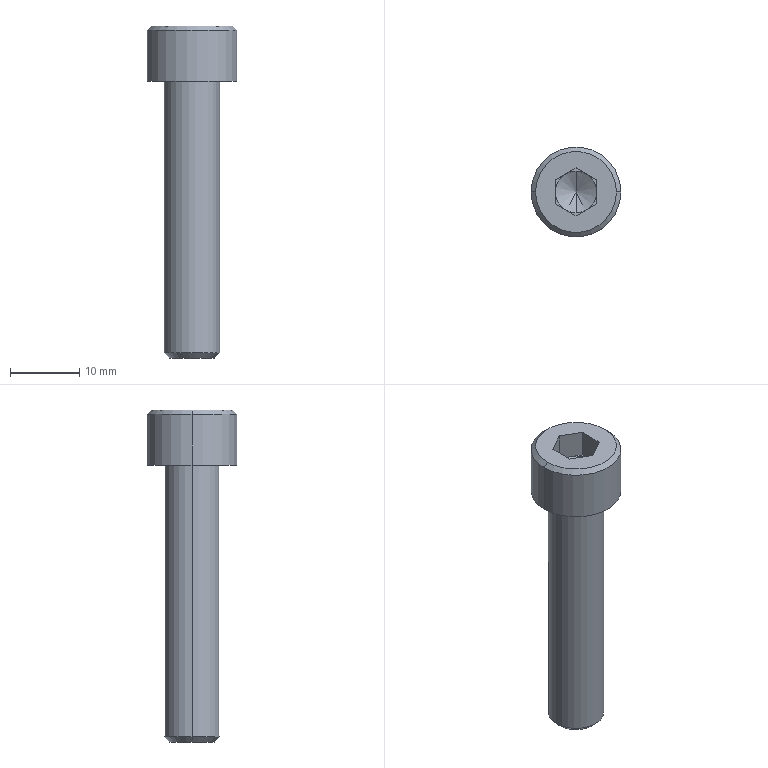Part | SolidWorks | features Chamfer 2, ICE 2, RevCut 1, Revolution 1 | 1 solid | 25 faces | box 13 x 13 x 48 mm | volume 2916 mm3 | plane 15 | cone 6 | cylinder 4 | commonest cylinder face diameters 8 x2 13 x2
STEP:
#1=CARTESIAN_POINT('',(-3.233,0.,-40.));
#2=VERTEX_POINT('',#1);
#3=CARTESIAN_POINT('',(3.233,0.,-40.));
#4=VERTEX_POINT('',#3);
#5=CARTESIAN_POINT('',(0.,0.,-40.));
#6=DIRECTION('',(0.,0.,-1.));
#7=DIRECTION('',(-1.,0.,0.));
#8=AXIS2_PLACEMENT_3D('',#5,#6,#7);
#9=CIRCLE('',#8,3.233);
#10=EDGE_CURVE('',#2,#4,#9,.T.);
#11=ORIENTED_EDGE('',*,*,#10,.F.);
#12=CARTESIAN_POINT('',(-4.,0.,-39.233));
#13=VERTEX_POINT('',#12);
#14=CARTESIAN_POINT('',(-3.233,0.,-40.));
#15=DIRECTION('',(-0.7071,0.,0.7071));
#16=VECTOR('',#15,1000.);
#17=LINE('',#14,#16);
#18=EDGE_CURVE('',#2,#13,#17,.T.);
#19=ORIENTED_EDGE('',*,*,#18,.T.);
#20=CARTESIAN_POINT('',(4.,0.,-39.233));
#21=VERTEX_POINT('',#20);
#22=CARTESIAN_POINT('',(0.,0.,-39.233));
#23=DIRECTION('',(0.,0.,1.));
#24=DIRECTION('',(-1.,0.,0.));
#25=AXIS2_PLACEMENT_3D('',#22,#23,#24);
#26=CIRCLE('',#25,4.);
#27=EDGE_CURVE('',#21,#13,#26,.T.);
#28=ORIENTED_EDGE('',*,*,#27,.F.);
#29=CARTESIAN_POINT('',(3.233,0.,-40.));
#30=DIRECTION('',(0.7071,0.,0.7071));
#31=VECTOR('',#30,1000.);
#32=LINE('',#29,#31);
#33=EDGE_CURVE('',#4,#21,#32,.T.);
#34=ORIENTED_EDGE('',*,*,#33,.F.);
#35=EDGE_LOOP('',(#11,#19,#28,#34));
#36=FACE_OUTER_BOUND('',#35,.T.);
#37=CARTESIAN_POINT('',(0.,0.,-40.));
#38=DIRECTION('',(0.,0.,1.));
#39=DIRECTION('',(1.,0.,0.));
#40=AXIS2_PLACEMENT_3D('',#37,#38,#39);
#41=CONICAL_SURFACE('',#40,3.233,0.7854);
#42=ADVANCED_FACE('',(#36),#41,.T.);
#43=CARTESIAN_POINT('',(5.85,0.,8.));
#44=VERTEX_POINT('',#43);
#45=CARTESIAN_POINT('',(-5.85,0.,8.));
#46=VERTEX_POINT('',#45);
#47=CARTESIAN_POINT('',(0.,0.,8.));
#48=DIRECTION('',(0.,0.,1.));
#49=DIRECTION('',(1.,0.,0.));
#50=AXIS2_PLACEMENT_3D('',#47,#48,#49);
#51=CIRCLE('',#50,5.85);
#52=EDGE_CURVE('',#44,#46,#51,.T.);
#53=ORIENTED_EDGE('',*,*,#52,.F.);
#54=CARTESIAN_POINT('',(6.5,0.,7.35));
#55=VERTEX_POINT('',#54);
#56=CARTESIAN_POINT('',(5.85,0.,8.));
#57=DIRECTION('',(0.7071,0.,-0.7071));
#58=VECTOR('',#57,1000.);
#59=LINE('',#56,#58);
#60=EDGE_CURVE('',#44,#55,#59,.T.);
#61=ORIENTED_EDGE('',*,*,#60,.T.);
#62=CARTESIAN_POINT('',(-6.5,0.,7.35));
#63=VERTEX_POINT('',#62);
#64=CARTESIAN_POINT('',(0.,0.,7.35));
#65=DIRECTION('',(0.,0.,-1.));
#66=DIRECTION('',(1.,0.,0.));
#67=AXIS2_PLACEMENT_3D('',#64,#65,#66);
#68=CIRCLE('',#67,6.5);
#69=EDGE_CURVE('',#63,#55,#68,.T.);
#70=ORIENTED_EDGE('',*,*,#69,.F.);
#71=CARTESIAN_POINT('',(-5.85,0.,8.));
#72=DIRECTION('',(-0.7071,0.,-0.7071));
#73=VECTOR('',#72,1000.);
#74=LINE('',#71,#73);
#75=EDGE_CURVE('',#46,#63,#74,.T.);
#76=ORIENTED_EDGE('',*,*,#75,.F.);
#77=EDGE_LOOP('',(#53,#61,#70,#76));
#78=FACE_OUTER_BOUND('',#77,.T.);
#79=CARTESIAN_POINT('',(0.,0.,8.));
#80=DIRECTION('',(0.,0.,-1.));
#81=DIRECTION('',(-1.,0.,0.));
#82=AXIS2_PLACEMENT_3D('',#79,#80,#81);
#83=CONICAL_SURFACE('',#82,5.85,0.7854);
#84=ADVANCED_FACE('',(#78),#83,.T.);
#85=CARTESIAN_POINT('',(0.,0.,2.268));
#86=VERTEX_POINT('',#85);
#87=CARTESIAN_POINT('',(0.,-3.,4.));
#88=VERTEX_POINT('',#87);
#89=CARTESIAN_POINT('',(0.,0.,2.268));
#90=DIRECTION('',(0.,-0.866,0.5));
#91=VECTOR('',#90,1000.);
#92=LINE('',#89,#91);
#93=EDGE_CURVE('',#86,#88,#92,.T.);
#94=ORIENTED_EDGE('',*,*,#93,.F.);
#95=CARTESIAN_POINT('',(0.,3.,4.));
#96=VERTEX_POINT('',#95);
#97=CARTESIAN_POINT('',(0.,0.,2.268));
#98=DIRECTION('',(0.,0.866,0.5));
#99=VECTOR('',#98,1000.);
#100=LINE('',#97,#99);
#101=EDGE_CURVE('',#86,#96,#100,.T.);
#102=ORIENTED_EDGE('',*,*,#101,.T.);
#103=CARTESIAN_POINT('',(-1.5,2.598,4.));
#104=VERTEX_POINT('',#103);
#105=CARTESIAN_POINT('',(0.,0.,4.));
#106=DIRECTION('',(0.,0.,-1.));
#107=DIRECTION('',(0.,1.,0.));
#108=AXIS2_PLACEMENT_3D('',#105,#106,#107);
#109=CIRCLE('',#108,3.);
#110=EDGE_CURVE('',#104,#96,#109,.T.);
#111=ORIENTED_EDGE('',*,*,#110,.F.);
#112=CARTESIAN_POINT('',(-3.,0.,4.));
#113=VERTEX_POINT('',#112);
#114=CARTESIAN_POINT('',(0.,0.,4.));
#115=DIRECTION('',(0.,0.,-1.));
#116=DIRECTION('',(0.,1.,0.));
#117=AXIS2_PLACEMENT_3D('',#114,#115,#116);
#118=CIRCLE('',#117,3.);
#119=EDGE_CURVE('',#113,#104,#118,.T.);
#120=ORIENTED_EDGE('',*,*,#119,.F.);
#121=CARTESIAN_POINT('',(-1.5,-2.598,4.));
#122=VERTEX_POINT('',#121);
#123=CARTESIAN_POINT('',(0.,0.,4.));
#124=DIRECTION('',(0.,0.,-1.));
#125=DIRECTION('',(0.,1.,0.));
#126=AXIS2_PLACEMENT_3D('',#123,#124,#125);
#127=CIRCLE('',#126,3.);
#128=EDGE_CURVE('',#122,#113,#127,.T.);
#129=ORIENTED_EDGE('',*,*,#128,.F.);
#130=CARTESIAN_POINT('',(0.,0.,4.));
#131=DIRECTION('',(0.,0.,-1.));
#132=DIRECTION('',(0.,1.,0.));
#133=AXIS2_PLACEMENT_3D('',#130,#131,#132);
#134=CIRCLE('',#133,3.);
#135=EDGE_CURVE('',#88,#122,#134,.T.);
#136=ORIENTED_EDGE('',*,*,#135,.F.);
#137=EDGE_LOOP('',(#94,#102,#111,#120,#129,#136));
#138=FACE_OUTER_BOUND('',#137,.T.);
#139=CARTESIAN_POINT('',(0.,0.,1002.268));
#140=DIRECTION('',(0.,0.,1.));
#141=DIRECTION('',(0.,-1.,0.));
#142=AXIS2_PLACEMENT_3D('',#139,#140,#141);
#143=CONICAL_SURFACE('',#142,1732.051,1.047);
#144=ADVANCED_FACE('',(#138),#143,.F.);
#145=ORIENTED_EDGE('',*,*,#27,.T.);
#146=CARTESIAN_POINT('',(-4.,0.,0.));
#147=VERTEX_POINT('',#146);
#148=CARTESIAN_POINT('',(-4.,0.,-40.));
#149=DIRECTION('',(0.,0.,1.));
#150=VECTOR('',#149,1000.);
#151=LINE('',#148,#150);
#152=EDGE_CURVE('',#13,#147,#151,.T.);
#153=ORIENTED_EDGE('',*,*,#152,.T.);
#154=CARTESIAN_POINT('',(4.,0.,0.));
#155=VERTEX_POINT('',#154);
#156=CARTESIAN_POINT('',(0.,0.,0.));
#157=DIRECTION('',(0.,0.,-1.));
#158=DIRECTION('',(-1.,0.,0.));
#159=AXIS2_PLACEMENT_3D('',#156,#157,#158);
#160=CIRCLE('',#159,4.);
#161=EDGE_CURVE('',#147,#155,#160,.T.);
#162=ORIENTED_EDGE('',*,*,#161,.T.);
#163=CARTESIAN_POINT('',(4.,0.,-40.));
#164=DIRECTION('',(0.,0.,1.));
#165=VECTOR('',#164,1000.);
#166=LINE('',#163,#165);
#167=EDGE_CURVE('',#21,#155,#166,.T.);
#168=ORIENTED_EDGE('',*,*,#167,.F.);
#169=EDGE_LOOP('',(#145,#153,#162,#168));
#170=FACE_OUTER_BOUND('',#169,.T.);
#171=CARTESIAN_POINT('',(0.,0.,-40.));
#172=DIRECTION('',(0.,0.,1.));
#173=DIRECTION('',(1.,0.,0.));
#174=AXIS2_PLACEMENT_3D('',#171,#172,#173);
#175=CYLINDRICAL_SURFACE('',#174,4.);
#176=ADVANCED_FACE('',(#170),#175,.T.);
#177=CARTESIAN_POINT('',(6.5,0.,0.));
#178=VERTEX_POINT('',#177);
#179=CARTESIAN_POINT('',(-6.5,0.,0.));
#180=VERTEX_POINT('',#179);
#181=CARTESIAN_POINT('',(0.,0.,0.));
#182=DIRECTION('',(0.,0.,1.));
#183=DIRECTION('',(1.,0.,0.));
#184=AXIS2_PLACEMENT_3D('',#181,#182,#183);
#185=CIRCLE('',#184,6.5);
#186=EDGE_CURVE('',#178,#180,#185,.T.);
#187=ORIENTED_EDGE('',*,*,#186,.T.);
#188=CARTESIAN_POINT('',(-6.5,0.,0.));
#189=DIRECTION('',(0.,0.,1.));
#190=VECTOR('',#189,1000.);
#191=LINE('',#188,#190);
#192=EDGE_CURVE('',#180,#63,#191,.T.);
#193=ORIENTED_EDGE('',*,*,#192,.T.);
#194=ORIENTED_EDGE('',*,*,#69,.T.);
#195=CARTESIAN_POINT('',(6.5,0.,0.));
#196=DIRECTION('',(0.,0.,1.));
#197=VECTOR('',#196,1000.);
#198=LINE('',#195,#197);
#199=EDGE_CURVE('',#178,#55,#198,.T.);
#200=ORIENTED_EDGE('',*,*,#199,.F.);
#201=EDGE_LOOP('',(#187,#193,#194,#200));
#202=FACE_OUTER_BOUND('',#201,.T.);
#203=CARTESIAN_POINT('',(0.,0.,0.));
#204=DIRECTION('',(0.,0.,1.));
#205=DIRECTION('',(1.,0.,0.));
#206=AXIS2_PLACEMENT_3D('',#203,#204,#205);
#207=CYLINDRICAL_SURFACE('',#206,6.5);
#208=ADVANCED_FACE('',(#202),#207,.T.);
#209=CARTESIAN_POINT('',(3.,1.732,4.));
#210=VERTEX_POINT('',#209);
#211=CARTESIAN_POINT('',(1.5,2.598,4.));
#212=VERTEX_POINT('',#211);
#213=CARTESIAN_POINT('',(3.,1.732,4.));
#214=DIRECTION('',(-0.866,0.5,0.));
#215=VECTOR('',#214,1000.);
#216=LINE('',#213,#215);
#217=EDGE_CURVE('',#210,#212,#216,.T.);
#218=ORIENTED_EDGE('',*,*,#217,.T.);
#219=CARTESIAN_POINT('',(3.,0.,4.));
#220=VERTEX_POINT('',#219);
#221=CARTESIAN_POINT('',(0.,0.,4.));
#222=DIRECTION('',(0.,0.,-1.));
#223=DIRECTION('',(0.,1.,0.));
#224=AXIS2_PLACEMENT_3D('',#221,#222,#223);
#225=CIRCLE('',#224,3.);
#226=EDGE_CURVE('',#212,#220,#225,.T.);
#227=ORIENTED_EDGE('',*,*,#226,.T.);
#228=CARTESIAN_POINT('',(3.,-1.732,4.));
#229=DIRECTION('',(0.,1.,0.));
#230=VECTOR('',#229,1000.);
#231=LINE('',#228,#230);
#232=EDGE_CURVE('',#220,#210,#231,.T.);
#233=ORIENTED_EDGE('',*,*,#232,.T.);
#234=EDGE_LOOP('',(#218,#227,#233));
#235=FACE_OUTER_BOUND('',#234,.T.);
#236=CARTESIAN_POINT('',(0.,0.,4.));
#237=DIRECTION('',(0.,0.,1.));
#238=DIRECTION('',(1.,0.,0.));
#239=AXIS2_PLACEMENT_3D('',#236,#237,#238);
#240=PLANE('',#239);
#241=ADVANCED_FACE('',(#235),#240,.T.);
#242=CARTESIAN_POINT('',(3.,-1.732,4.));
#243=VERTEX_POINT('',#242);
#244=CARTESIAN_POINT('',(3.,-1.732,4.));
#245=DIRECTION('',(0.,1.,0.));
#246=VECTOR('',#245,1000.);
#247=LINE('',#244,#246);
#248=EDGE_CURVE('',#243,#220,#247,.T.);
#249=ORIENTED_EDGE('',*,*,#248,.T.);
#250=CARTESIAN_POINT('',(1.5,-2.598,4.));
#251=VERTEX_POINT('',#250);
#252=CARTESIAN_POINT('',(0.,0.,4.));
#253=DIRECTION('',(0.,0.,-1.));
#254=DIRECTION('',(0.,1.,0.));
#255=AXIS2_PLACEMENT_3D('',#252,#253,#254);
#256=CIRCLE('',#255,3.);
#257=EDGE_CURVE('',#220,#251,#256,.T.);
#258=ORIENTED_EDGE('',*,*,#257,.T.);
#259=CARTESIAN_POINT('',(0.,-3.464,4.));
#260=DIRECTION('',(0.866,0.5,0.));
#261=VECTOR('',#260,1000.);
#262=LINE('',#259,#261);
#263=EDGE_CURVE('',#251,#243,#262,.T.);
#264=ORIENTED_EDGE('',*,*,#263,.T.);
#265=EDGE_LOOP('',(#249,#258,#264));
#266=FACE_OUTER_BOUND('',#265,.T.);
#267=CARTESIAN_POINT('',(0.,0.,4.));
#268=DIRECTION('',(0.,0.,1.));
#269=DIRECTION('',(1.,0.,0.));
#270=AXIS2_PLACEMENT_3D('',#267,#268,#269);
#271=PLANE('',#270);
#272=ADVANCED_FACE('',(#266),#271,.T.);
#273=CARTESIAN_POINT('',(0.,-3.464,4.));
#274=VERTEX_POINT('',#273);
#275=CARTESIAN_POINT('',(0.,-3.464,4.));
#276=DIRECTION('',(0.866,0.5,0.));
#277=VECTOR('',#276,1000.);
#278=LINE('',#275,#277);
#279=EDGE_CURVE('',#274,#251,#278,.T.);
#280=ORIENTED_EDGE('',*,*,#279,.T.);
#281=CARTESIAN_POINT('',(0.,0.,4.));
#282=DIRECTION('',(0.,0.,-1.));
#283=DIRECTION('',(0.,1.,0.));
#284=AXIS2_PLACEMENT_3D('',#281,#282,#283);
#285=CIRCLE('',#284,3.);
#286=EDGE_CURVE('',#251,#88,#285,.T.);
#287=ORIENTED_EDGE('',*,*,#286,.T.);
#288=ORIENTED_EDGE('',*,*,#135,.T.);
#289=CARTESIAN_POINT('',(-3.,-1.732,4.));
#290=DIRECTION('',(0.866,-0.5,0.));
#291=VECTOR('',#290,1000.);
#292=LINE('',#289,#291);
#293=EDGE_CURVE('',#122,#274,#292,.T.);
#294=ORIENTED_EDGE('',*,*,#293,.T.);
#295=EDGE_LOOP('',(#280,#287,#288,#294));
#296=FACE_OUTER_BOUND('',#295,.T.);
#297=CARTESIAN_POINT('',(0.,0.,4.));
#298=DIRECTION('',(0.,0.,1.));
#299=DIRECTION('',(1.,0.,0.));
#300=AXIS2_PLACEMENT_3D('',#297,#298,#299);
#301=PLANE('',#300);
#302=ADVANCED_FACE('',(#296),#301,.T.);
#303=CARTESIAN_POINT('',(-3.,-1.732,4.));
#304=VERTEX_POINT('',#303);
#305=CARTESIAN_POINT('',(-3.,-1.732,4.));
#306=DIRECTION('',(0.866,-0.5,0.));
#307=VECTOR('',#306,1000.);
#308=LINE('',#305,#307);
#309=EDGE_CURVE('',#304,#122,#308,.T.);
#310=ORIENTED_EDGE('',*,*,#309,.T.);
#311=ORIENTED_EDGE('',*,*,#128,.T.);
#312=CARTESIAN_POINT('',(-3.,1.732,4.));
#313=DIRECTION('',(0.,-1.,0.));
#314=VECTOR('',#313,1000.);
#315=LINE('',#312,#314);
#316=EDGE_CURVE('',#113,#304,#315,.T.);
#317=ORIENTED_EDGE('',*,*,#316,.T.);
#318=EDGE_LOOP('',(#310,#311,#317));
#319=FACE_OUTER_BOUND('',#318,.T.);
#320=CARTESIAN_POINT('',(0.,0.,4.));
#321=DIRECTION('',(0.,0.,1.));
#322=DIRECTION('',(1.,0.,0.));
#323=AXIS2_PLACEMENT_3D('',#320,#321,#322);
#324=PLANE('',#323);
#325=ADVANCED_FACE('',(#319),#324,.T.);
#326=CARTESIAN_POINT('',(-3.,1.732,4.));
#327=VERTEX_POINT('',#326);
#328=CARTESIAN_POINT('',(-3.,1.732,4.));
#329=DIRECTION('',(0.,-1.,0.));
#330=VECTOR('',#329,1000.);
#331=LINE('',#328,#330);
#332=EDGE_CURVE('',#327,#113,#331,.T.);
#333=ORIENTED_EDGE('',*,*,#332,.T.);
#334=ORIENTED_EDGE('',*,*,#119,.T.);
#335=CARTESIAN_POINT('',(0.,3.464,4.));
#336=DIRECTION('',(-0.866,-0.5,0.));
#337=VECTOR('',#336,1000.);
#338=LINE('',#335,#337);
#339=EDGE_CURVE('',#104,#327,#338,.T.);
#340=ORIENTED_EDGE('',*,*,#339,.T.);
#341=EDGE_LOOP('',(#333,#334,#340));
#342=FACE_OUTER_BOUND('',#341,.T.);
#343=CARTESIAN_POINT('',(0.,0.,4.));
#344=DIRECTION('',(0.,0.,1.));
#345=DIRECTION('',(1.,0.,0.));
#346=AXIS2_PLACEMENT_3D('',#343,#344,#345);
#347=PLANE('',#346);
#348=ADVANCED_FACE('',(#342),#347,.T.);
#349=CARTESIAN_POINT('',(0.,3.464,4.));
#350=VERTEX_POINT('',#349);
#351=CARTESIAN_POINT('',(0.,3.464,4.));
#352=DIRECTION('',(-0.866,-0.5,0.));
#353=VECTOR('',#352,1000.);
#354=LINE('',#351,#353);
#355=EDGE_CURVE('',#350,#104,#354,.T.);
#356=ORIENTED_EDGE('',*,*,#355,.T.);
#357=ORIENTED_EDGE('',*,*,#110,.T.);
#358=CARTESIAN_POINT('',(0.,0.,4.));
#359=DIRECTION('',(0.,0.,-1.));
#360=DIRECTION('',(0.,1.,0.));
#361=AXIS2_PLACEMENT_3D('',#358,#359,#360);
#362=CIRCLE('',#361,3.);
#363=EDGE_CURVE('',#96,#212,#362,.T.);
#364=ORIENTED_EDGE('',*,*,#363,.T.);
#365=CARTESIAN_POINT('',(3.,1.732,4.));
#366=DIRECTION('',(-0.866,0.5,0.));
#367=VECTOR('',#366,1000.);
#368=LINE('',#365,#367);
#369=EDGE_CURVE('',#212,#350,#368,.T.);
#370=ORIENTED_EDGE('',*,*,#369,.T.);
#371=EDGE_LOOP('',(#356,#357,#364,#370));
#372=FACE_OUTER_BOUND('',#371,.T.);
#373=CARTESIAN_POINT('',(0.,0.,4.));
#374=DIRECTION('',(0.,0.,1.));
#375=DIRECTION('',(1.,0.,0.));
#376=AXIS2_PLACEMENT_3D('',#373,#374,#375);
#377=PLANE('',#376);
#378=ADVANCED_FACE('',(#372),#377,.T.);
#379=ORIENTED_EDGE('',*,*,#186,.F.);
#380=CARTESIAN_POINT('',(0.,0.,0.));
#381=DIRECTION('',(0.,0.,1.));
#382=DIRECTION('',(1.,0.,0.));
#383=AXIS2_PLACEMENT_3D('',#380,#381,#382);
#384=CIRCLE('',#383,6.5);
#385=EDGE_CURVE('',#180,#178,#384,.T.);
#386=ORIENTED_EDGE('',*,*,#385,.F.);
#387=EDGE_LOOP('',(#379,#386));
#388=FACE_OUTER_BOUND('',#387,.T.);
#389=CARTESIAN_POINT('',(0.,0.,0.));
#390=DIRECTION('',(0.,0.,-1.));
#391=DIRECTION('',(-1.,0.,0.));
#392=AXIS2_PLACEMENT_3D('',#389,#390,#391);
#393=CIRCLE('',#392,4.);
#394=EDGE_CURVE('',#155,#147,#393,.T.);
#395=ORIENTED_EDGE('',*,*,#394,.F.);
#396=ORIENTED_EDGE('',*,*,#161,.F.);
#397=EDGE_LOOP('',(#395,#396));
#398=FACE_BOUND('',#397,.T.);
#399=CARTESIAN_POINT('',(6.5,0.,0.));
#400=DIRECTION('',(0.,0.,-1.));
#401=DIRECTION('',(-1.,0.,0.));
#402=AXIS2_PLACEMENT_3D('',#399,#400,#401);
#403=PLANE('',#402);
#404=ADVANCED_FACE('',(#388,#398),#403,.T.);
#405=ORIENTED_EDGE('',*,*,#192,.F.);
#406=ORIENTED_EDGE('',*,*,#385,.T.);
#407=ORIENTED_EDGE('',*,*,#199,.T.);
#408=CARTESIAN_POINT('',(0.,0.,7.35));
#409=DIRECTION('',(0.,0.,-1.));
#410=DIRECTION('',(1.,0.,0.));
#411=AXIS2_PLACEMENT_3D('',#408,#409,#410);
#412=CIRCLE('',#411,6.5);
#413=EDGE_CURVE('',#55,#63,#412,.T.);
#414=ORIENTED_EDGE('',*,*,#413,.T.);
#415=EDGE_LOOP('',(#405,#406,#407,#414));
#416=FACE_OUTER_BOUND('',#415,.T.);
#417=CARTESIAN_POINT('',(0.,0.,0.));
#418=DIRECTION('',(0.,0.,1.));
#419=DIRECTION('',(1.,0.,0.));
#420=AXIS2_PLACEMENT_3D('',#417,#418,#419);
#421=CYLINDRICAL_SURFACE('',#420,6.5);
#422=ADVANCED_FACE('',(#416),#421,.T.);
#423=CARTESIAN_POINT('',(0.,0.,8.));
#424=DIRECTION('',(0.,0.,1.));
#425=DIRECTION('',(1.,0.,0.));
#426=AXIS2_PLACEMENT_3D('',#423,#424,#425);
#427=CIRCLE('',#426,5.85);
#428=EDGE_CURVE('',#46,#44,#427,.T.);
#429=ORIENTED_EDGE('',*,*,#428,.T.);
#430=ORIENTED_EDGE('',*,*,#52,.T.);
#431=EDGE_LOOP('',(#429,#430));
#432=FACE_OUTER_BOUND('',#431,.T.);
#433=CARTESIAN_POINT('',(3.,-1.732,8.));
#434=VERTEX_POINT('',#433);
#435=CARTESIAN_POINT('',(3.,1.732,8.));
#436=VERTEX_POINT('',#435);
#437=CARTESIAN_POINT('',(3.,-1.732,8.));
#438=DIRECTION('',(0.,1.,0.));
#439=VECTOR('',#438,1000.);
#440=LINE('',#437,#439);
#441=EDGE_CURVE('',#434,#436,#440,.T.);
#442=ORIENTED_EDGE('',*,*,#441,.F.);
#443=CARTESIAN_POINT('',(0.,-3.464,8.));
#444=VERTEX_POINT('',#443);
#445=CARTESIAN_POINT('',(0.,-3.464,8.));
#446=DIRECTION('',(0.866,0.5,0.));
#447=VECTOR('',#446,1000.);
#448=LINE('',#445,#447);
#449=EDGE_CURVE('',#444,#434,#448,.T.);
#450=ORIENTED_EDGE('',*,*,#449,.F.);
#451=CARTESIAN_POINT('',(-3.,-1.732,8.));
#452=VERTEX_POINT('',#451);
#453=CARTESIAN_POINT('',(-3.,-1.732,8.));
#454=DIRECTION('',(0.866,-0.5,0.));
#455=VECTOR('',#454,1000.);
#456=LINE('',#453,#455);
#457=EDGE_CURVE('',#452,#444,#456,.T.);
#458=ORIENTED_EDGE('',*,*,#457,.F.);
#459=CARTESIAN_POINT('',(-3.,1.732,8.));
#460=VERTEX_POINT('',#459);
#461=CARTESIAN_POINT('',(-3.,1.732,8.));
#462=DIRECTION('',(0.,-1.,0.));
#463=VECTOR('',#462,1000.);
#464=LINE('',#461,#463);
#465=EDGE_CURVE('',#460,#452,#464,.T.);
#466=ORIENTED_EDGE('',*,*,#465,.F.);
#467=CARTESIAN_POINT('',(0.,3.464,8.));
#468=VERTEX_POINT('',#467);
#469=CARTESIAN_POINT('',(0.,3.464,8.));
#470=DIRECTION('',(-0.866,-0.5,0.));
#471=VECTOR('',#470,1000.);
#472=LINE('',#469,#471);
#473=EDGE_CURVE('',#468,#460,#472,.T.);
#474=ORIENTED_EDGE('',*,*,#473,.F.);
#475=CARTESIAN_POINT('',(3.,1.732,8.));
#476=DIRECTION('',(-0.866,0.5,0.));
#477=VECTOR('',#476,1000.);
#478=LINE('',#475,#477);
#479=EDGE_CURVE('',#436,#468,#478,.T.);
#480=ORIENTED_EDGE('',*,*,#479,.F.);
#481=EDGE_LOOP('',(#442,#450,#458,#466,#474,#480));
#482=FACE_BOUND('',#481,.T.);
#483=CARTESIAN_POINT('',(0.,0.,8.));
#484=DIRECTION('',(0.,0.,1.));
#485=DIRECTION('',(1.,0.,0.));
#486=AXIS2_PLACEMENT_3D('',#483,#484,#485);
#487=PLANE('',#486);
#488=ADVANCED_FACE('',(#432,#482),#487,.T.);
#489=ORIENTED_EDGE('',*,*,#152,.F.);
#490=CARTESIAN_POINT('',(0.,0.,-39.233));
#491=DIRECTION('',(0.,0.,1.));
#492=DIRECTION('',(-1.,0.,0.));
#493=AXIS2_PLACEMENT_3D('',#490,#491,#492);
#494=CIRCLE('',#493,4.);
#495=EDGE_CURVE('',#13,#21,#494,.T.);
#496=ORIENTED_EDGE('',*,*,#495,.T.);
#497=ORIENTED_EDGE('',*,*,#167,.T.);
#498=ORIENTED_EDGE('',*,*,#394,.T.);
#499=EDGE_LOOP('',(#489,#496,#497,#498));
#500=FACE_OUTER_BOUND('',#499,.T.);
#501=CARTESIAN_POINT('',(0.,0.,-40.));
#502=DIRECTION('',(0.,0.,1.));
#503=DIRECTION('',(1.,0.,0.));
#504=AXIS2_PLACEMENT_3D('',#501,#502,#503);
#505=CYLINDRICAL_SURFACE('',#504,4.);
#506=ADVANCED_FACE('',(#500),#505,.T.);
#507=CARTESIAN_POINT('',(0.,0.,-40.));
#508=DIRECTION('',(0.,0.,-1.));
#509=DIRECTION('',(-1.,0.,0.));
#510=AXIS2_PLACEMENT_3D('',#507,#508,#509);
#511=CIRCLE('',#510,3.233);
#512=EDGE_CURVE('',#4,#2,#511,.T.);
#513=ORIENTED_EDGE('',*,*,#512,.T.);
#514=ORIENTED_EDGE('',*,*,#10,.T.);
#515=EDGE_LOOP('',(#513,#514));
#516=FACE_OUTER_BOUND('',#515,.T.);
#517=CARTESIAN_POINT('',(0.,0.,-40.));
#518=DIRECTION('',(0.,0.,-1.));
#519=DIRECTION('',(-1.,0.,0.));
#520=AXIS2_PLACEMENT_3D('',#517,#518,#519);
#521=PLANE('',#520);
#522=ADVANCED_FACE('',(#516),#521,.T.);
#523=ORIENTED_EDGE('',*,*,#441,.T.);
#524=CARTESIAN_POINT('',(3.,1.732,4.));
#525=DIRECTION('',(0.,0.,1.));
#526=VECTOR('',#525,1000.);
#527=LINE('',#524,#526);
#528=EDGE_CURVE('',#210,#436,#527,.T.);
#529=ORIENTED_EDGE('',*,*,#528,.F.);
#530=ORIENTED_EDGE('',*,*,#232,.F.);
#531=ORIENTED_EDGE('',*,*,#248,.F.);
#532=CARTESIAN_POINT('',(3.,-1.732,4.));
#533=DIRECTION('',(0.,0.,1.));
#534=VECTOR('',#533,1000.);
#535=LINE('',#532,#534);
#536=EDGE_CURVE('',#243,#434,#535,.T.);
#537=ORIENTED_EDGE('',*,*,#536,.T.);
#538=EDGE_LOOP('',(#523,#529,#530,#531,#537));
#539=FACE_OUTER_BOUND('',#538,.T.);
#540=CARTESIAN_POINT('',(3.,-1.732,4.));
#541=DIRECTION('',(1.,0.,0.));
#542=DIRECTION('',(0.,1.,0.));
#543=AXIS2_PLACEMENT_3D('',#540,#541,#542);
#544=PLANE('',#543);
#545=ADVANCED_FACE('',(#539),#544,.F.);
#546=ORIENTED_EDGE('',*,*,#449,.T.);
#547=ORIENTED_EDGE('',*,*,#536,.F.);
#548=ORIENTED_EDGE('',*,*,#263,.F.);
#549=ORIENTED_EDGE('',*,*,#279,.F.);
#550=CARTESIAN_POINT('',(0.,-3.464,4.));
#551=DIRECTION('',(0.,0.,1.));
#552=VECTOR('',#551,1000.);
#553=LINE('',#550,#552);
#554=EDGE_CURVE('',#274,#444,#553,.T.);
#555=ORIENTED_EDGE('',*,*,#554,.T.);
#556=EDGE_LOOP('',(#546,#547,#548,#549,#555));
#557=FACE_OUTER_BOUND('',#556,.T.);
#558=CARTESIAN_POINT('',(0.,-3.464,4.));
#559=DIRECTION('',(0.5,-0.866,0.));
#560=DIRECTION('',(0.866,0.5,0.));
#561=AXIS2_PLACEMENT_3D('',#558,#559,#560);
#562=PLANE('',#561);
#563=ADVANCED_FACE('',(#557),#562,.F.);
#564=ORIENTED_EDGE('',*,*,#457,.T.);
#565=ORIENTED_EDGE('',*,*,#554,.F.);
#566=ORIENTED_EDGE('',*,*,#293,.F.);
#567=ORIENTED_EDGE('',*,*,#309,.F.);
#568=CARTESIAN_POINT('',(-3.,-1.732,4.));
#569=DIRECTION('',(0.,0.,1.));
#570=VECTOR('',#569,1000.);
#571=LINE('',#568,#570);
#572=EDGE_CURVE('',#304,#452,#571,.T.);
#573=ORIENTED_EDGE('',*,*,#572,.T.);
#574=EDGE_LOOP('',(#564,#565,#566,#567,#573));
#575=FACE_OUTER_BOUND('',#574,.T.);
#576=CARTESIAN_POINT('',(-3.,-1.732,4.));
#577=DIRECTION('',(-0.5,-0.866,0.));
#578=DIRECTION('',(0.866,-0.5,0.));
#579=AXIS2_PLACEMENT_3D('',#576,#577,#578);
#580=PLANE('',#579);
#581=ADVANCED_FACE('',(#575),#580,.F.);
#582=ORIENTED_EDGE('',*,*,#465,.T.);
#583=ORIENTED_EDGE('',*,*,#572,.F.);
#584=ORIENTED_EDGE('',*,*,#316,.F.);
#585=ORIENTED_EDGE('',*,*,#332,.F.);
#586=CARTESIAN_POINT('',(-3.,1.732,4.));
#587=DIRECTION('',(0.,0.,1.));
#588=VECTOR('',#587,1000.);
#589=LINE('',#586,#588);
#590=EDGE_CURVE('',#327,#460,#589,.T.);
#591=ORIENTED_EDGE('',*,*,#590,.T.);
#592=EDGE_LOOP('',(#582,#583,#584,#585,#591));
#593=FACE_OUTER_BOUND('',#592,.T.);
#594=CARTESIAN_POINT('',(-3.,1.732,4.));
#595=DIRECTION('',(-1.,0.,0.));
#596=DIRECTION('',(0.,-1.,0.));
#597=AXIS2_PLACEMENT_3D('',#594,#595,#596);
#598=PLANE('',#597);
#599=ADVANCED_FACE('',(#593),#598,.F.);
#600=ORIENTED_EDGE('',*,*,#473,.T.);
#601=ORIENTED_EDGE('',*,*,#590,.F.);
#602=ORIENTED_EDGE('',*,*,#339,.F.);
#603=ORIENTED_EDGE('',*,*,#355,.F.);
#604=CARTESIAN_POINT('',(0.,3.464,4.));
#605=DIRECTION('',(0.,0.,1.));
#606=VECTOR('',#605,1000.);
#607=LINE('',#604,#606);
#608=EDGE_CURVE('',#350,#468,#607,.T.);
#609=ORIENTED_EDGE('',*,*,#608,.T.);
#610=EDGE_LOOP('',(#600,#601,#602,#603,#609));
#611=FACE_OUTER_BOUND('',#610,.T.);
#612=CARTESIAN_POINT('',(0.,3.464,4.));
#613=DIRECTION('',(-0.5,0.866,0.));
#614=DIRECTION('',(-0.866,-0.5,0.));
#615=AXIS2_PLACEMENT_3D('',#612,#613,#614);
#616=PLANE('',#615);
#617=ADVANCED_FACE('',(#611),#616,.F.);
#618=ORIENTED_EDGE('',*,*,#479,.T.);
#619=ORIENTED_EDGE('',*,*,#608,.F.);
#620=ORIENTED_EDGE('',*,*,#369,.F.);
#621=ORIENTED_EDGE('',*,*,#217,.F.);
#622=ORIENTED_EDGE('',*,*,#528,.T.);
#623=EDGE_LOOP('',(#618,#619,#620,#621,#622));
#624=FACE_OUTER_BOUND('',#623,.T.);
#625=CARTESIAN_POINT('',(3.,1.732,4.));
#626=DIRECTION('',(0.5,0.866,0.));
#627=DIRECTION('',(-0.866,0.5,0.));
#628=AXIS2_PLACEMENT_3D('',#625,#626,#627);
#629=PLANE('',#628);
#630=ADVANCED_FACE('',(#624),#629,.F.);
#631=ORIENTED_EDGE('',*,*,#101,.F.);
#632=ORIENTED_EDGE('',*,*,#93,.T.);
#633=ORIENTED_EDGE('',*,*,#286,.F.);
#634=ORIENTED_EDGE('',*,*,#257,.F.);
#635=ORIENTED_EDGE('',*,*,#226,.F.);
#636=ORIENTED_EDGE('',*,*,#363,.F.);
#637=EDGE_LOOP('',(#631,#632,#633,#634,#635,#636));
#638=FACE_OUTER_BOUND('',#637,.T.);
#639=CARTESIAN_POINT('',(0.,0.,1002.268));
#640=DIRECTION('',(0.,0.,1.));
#641=DIRECTION('',(0.,-1.,0.));
#642=AXIS2_PLACEMENT_3D('',#639,#640,#641);
#643=CONICAL_SURFACE('',#642,1732.051,1.047);
#644=ADVANCED_FACE('',(#638),#643,.F.);
#645=ORIENTED_EDGE('',*,*,#60,.F.);
#646=ORIENTED_EDGE('',*,*,#428,.F.);
#647=ORIENTED_EDGE('',*,*,#75,.T.);
#648=ORIENTED_EDGE('',*,*,#413,.F.);
#649=EDGE_LOOP('',(#645,#646,#647,#648));
#650=FACE_OUTER_BOUND('',#649,.T.);
#651=CARTESIAN_POINT('',(0.,0.,8.));
#652=DIRECTION('',(0.,0.,-1.));
#653=DIRECTION('',(-1.,0.,0.));
#654=AXIS2_PLACEMENT_3D('',#651,#652,#653);
#655=CONICAL_SURFACE('',#654,5.85,0.7854);
#656=ADVANCED_FACE('',(#650),#655,.T.);
#657=ORIENTED_EDGE('',*,*,#18,.F.);
#658=ORIENTED_EDGE('',*,*,#512,.F.);
#659=ORIENTED_EDGE('',*,*,#33,.T.);
#660=ORIENTED_EDGE('',*,*,#495,.F.);
#661=EDGE_LOOP('',(#657,#658,#659,#660));
#662=FACE_OUTER_BOUND('',#661,.T.);
#663=CARTESIAN_POINT('',(0.,0.,-40.));
#664=DIRECTION('',(0.,0.,1.));
#665=DIRECTION('',(1.,0.,0.));
#666=AXIS2_PLACEMENT_3D('',#663,#664,#665);
#667=CONICAL_SURFACE('',#666,3.233,0.7854);
#668=ADVANCED_FACE('',(#662),#667,.T.);
#669=CLOSED_SHELL('',(#42,#84,#144,#176,#208,#241,#272,#302,#325,#348,#378,#404,#422,#488,#506,#522,#545,#563,#581,#599,#617,#630,#644,#656,#668));
#670=MANIFOLD_SOLID_BREP('',#669);
#671=CARTESIAN_POINT('',(0.,0.,0.));
#672=DIRECTION('',(0.,0.,1.));
#673=DIRECTION('',(1.,0.,0.));
#674=AXIS2_PLACEMENT_3D('',#671,#672,#673);
#675=(LENGTH_UNIT()NAMED_UNIT(*)SI_UNIT(.MILLI.,.METRE.));
#676=UNCERTAINTY_MEASURE_WITH_UNIT(LENGTH_MEASURE(0.00001),#675,'','');
#677=(NAMED_UNIT(*)PLANE_ANGLE_UNIT()SI_UNIT($,.RADIAN.));
#678=(NAMED_UNIT(*)SI_UNIT($,.STERADIAN.)SOLID_ANGLE_UNIT());
#679=(GEOMETRIC_REPRESENTATION_CONTEXT(3)GLOBAL_UNCERTAINTY_ASSIGNED_CONTEXT((#676))GLOBAL_UNIT_ASSIGNED_CONTEXT((#675,#677,#678))REPRESENTATION_CONTEXT('',''));
#680=ADVANCED_BREP_SHAPE_REPRESENTATION('',(#670,#674),#679);